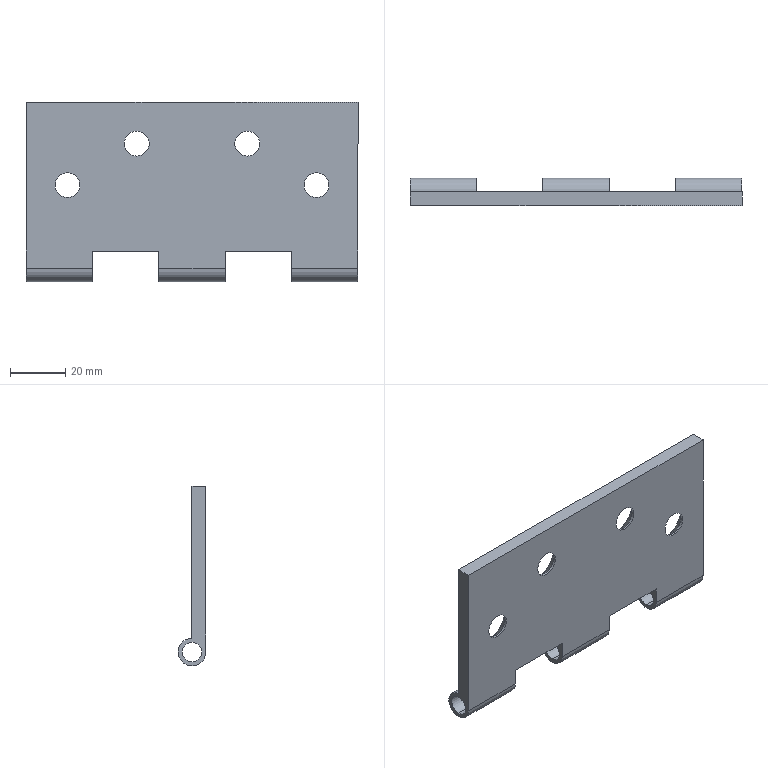Part | SolidWorks | features BaseBody 1 | 1 solid | 36 faces | box 120 x 10 x 65 mm | volume 33485 mm3 | cylinder 17 | plane 11 | cone 8 | commonest cylinder face diameters 9 x8 7 x6 10 x3
STEP:
#1=CARTESIAN_POINT('',(45.,0.85,-4.5));
#2=VERTEX_POINT('',#1);
#3=CARTESIAN_POINT('',(45.,0.85,4.5));
#4=VERTEX_POINT('',#3);
#5=CARTESIAN_POINT('',(45.,0.85,0.));
#6=DIRECTION('',(0.,1.,0.));
#7=DIRECTION('',(0.,0.,1.));
#8=AXIS2_PLACEMENT_3D('',#5,#6,#7);
#9=CIRCLE('',#8,4.5);
#10=EDGE_CURVE('',#2,#4,#9,.T.);
#11=ORIENTED_EDGE('',*,*,#10,.F.);
#12=CARTESIAN_POINT('',(45.,5.,-8.65));
#13=VERTEX_POINT('',#12);
#14=CARTESIAN_POINT('',(45.,5.,-8.65));
#15=DIRECTION('',(0.,0.7071,-0.7071));
#16=VECTOR('',#15,1000.);
#17=LINE('',#14,#16);
#18=EDGE_CURVE('',#2,#13,#17,.T.);
#19=ORIENTED_EDGE('',*,*,#18,.T.);
#20=CARTESIAN_POINT('',(45.,5.,8.65));
#21=VERTEX_POINT('',#20);
#22=CARTESIAN_POINT('',(45.,5.,0.));
#23=DIRECTION('',(0.,1.,0.));
#24=DIRECTION('',(0.,0.,1.));
#25=AXIS2_PLACEMENT_3D('',#22,#23,#24);
#26=CIRCLE('',#25,8.65);
#27=EDGE_CURVE('',#13,#21,#26,.T.);
#28=ORIENTED_EDGE('',*,*,#27,.T.);
#29=CARTESIAN_POINT('',(45.,5.,8.65));
#30=DIRECTION('',(0.,0.7071,0.7071));
#31=VECTOR('',#30,1000.);
#32=LINE('',#29,#31);
#33=EDGE_CURVE('',#4,#21,#32,.T.);
#34=ORIENTED_EDGE('',*,*,#33,.F.);
#35=EDGE_LOOP('',(#11,#19,#28,#34));
#36=FACE_OUTER_BOUND('',#35,.T.);
#37=CARTESIAN_POINT('',(45.,5.,0.));
#38=DIRECTION('',(0.,1.,0.));
#39=DIRECTION('',(0.,0.,1.));
#40=AXIS2_PLACEMENT_3D('',#37,#38,#39);
#41=CONICAL_SURFACE('',#40,8.65,0.7854);
#42=ADVANCED_FACE('',(#36),#41,.F.);
#43=CARTESIAN_POINT('',(45.,0.,-4.5));
#44=VERTEX_POINT('',#43);
#45=CARTESIAN_POINT('',(45.,0.,4.5));
#46=VERTEX_POINT('',#45);
#47=CARTESIAN_POINT('',(45.,0.,0.));
#48=DIRECTION('',(0.,1.,0.));
#49=DIRECTION('',(0.,0.,1.));
#50=AXIS2_PLACEMENT_3D('',#47,#48,#49);
#51=CIRCLE('',#50,4.5);
#52=EDGE_CURVE('',#44,#46,#51,.T.);
#53=ORIENTED_EDGE('',*,*,#52,.F.);
#54=CARTESIAN_POINT('',(45.,5.,-4.5));
#55=DIRECTION('',(0.,1.,0.));
#56=VECTOR('',#55,1000.);
#57=LINE('',#54,#56);
#58=EDGE_CURVE('',#44,#2,#57,.T.);
#59=ORIENTED_EDGE('',*,*,#58,.T.);
#60=ORIENTED_EDGE('',*,*,#10,.T.);
#61=CARTESIAN_POINT('',(45.,5.,4.5));
#62=DIRECTION('',(0.,1.,0.));
#63=VECTOR('',#62,1000.);
#64=LINE('',#61,#63);
#65=EDGE_CURVE('',#46,#4,#64,.T.);
#66=ORIENTED_EDGE('',*,*,#65,.F.);
#67=EDGE_LOOP('',(#53,#59,#60,#66));
#68=FACE_OUTER_BOUND('',#67,.T.);
#69=CARTESIAN_POINT('',(45.,5.,0.));
#70=DIRECTION('',(0.,1.,0.));
#71=DIRECTION('',(0.,0.,1.));
#72=AXIS2_PLACEMENT_3D('',#69,#70,#71);
#73=CYLINDRICAL_SURFACE('',#72,4.5);
#74=ADVANCED_FACE('',(#68),#73,.F.);
#75=CARTESIAN_POINT('',(20.,0.85,10.5));
#76=VERTEX_POINT('',#75);
#77=CARTESIAN_POINT('',(20.,0.85,19.5));
#78=VERTEX_POINT('',#77);
#79=CARTESIAN_POINT('',(20.,0.85,15.));
#80=DIRECTION('',(0.,1.,0.));
#81=DIRECTION('',(0.,0.,1.));
#82=AXIS2_PLACEMENT_3D('',#79,#80,#81);
#83=CIRCLE('',#82,4.5);
#84=EDGE_CURVE('',#76,#78,#83,.T.);
#85=ORIENTED_EDGE('',*,*,#84,.F.);
#86=CARTESIAN_POINT('',(20.,5.,6.35));
#87=VERTEX_POINT('',#86);
#88=CARTESIAN_POINT('',(20.,5.,6.35));
#89=DIRECTION('',(0.,0.7071,-0.7071));
#90=VECTOR('',#89,1000.);
#91=LINE('',#88,#90);
#92=EDGE_CURVE('',#76,#87,#91,.T.);
#93=ORIENTED_EDGE('',*,*,#92,.T.);
#94=CARTESIAN_POINT('',(20.,5.,23.65));
#95=VERTEX_POINT('',#94);
#96=CARTESIAN_POINT('',(20.,5.,15.));
#97=DIRECTION('',(0.,1.,0.));
#98=DIRECTION('',(0.,0.,1.));
#99=AXIS2_PLACEMENT_3D('',#96,#97,#98);
#100=CIRCLE('',#99,8.65);
#101=EDGE_CURVE('',#87,#95,#100,.T.);
#102=ORIENTED_EDGE('',*,*,#101,.T.);
#103=CARTESIAN_POINT('',(20.,5.,23.65));
#104=DIRECTION('',(0.,0.7071,0.7071));
#105=VECTOR('',#104,1000.);
#106=LINE('',#103,#105);
#107=EDGE_CURVE('',#78,#95,#106,.T.);
#108=ORIENTED_EDGE('',*,*,#107,.F.);
#109=EDGE_LOOP('',(#85,#93,#102,#108));
#110=FACE_OUTER_BOUND('',#109,.T.);
#111=CARTESIAN_POINT('',(20.,5.,15.));
#112=DIRECTION('',(0.,1.,0.));
#113=DIRECTION('',(0.,0.,1.));
#114=AXIS2_PLACEMENT_3D('',#111,#112,#113);
#115=CONICAL_SURFACE('',#114,8.65,0.7854);
#116=ADVANCED_FACE('',(#110),#115,.F.);
#117=CARTESIAN_POINT('',(20.,0.,10.5));
#118=VERTEX_POINT('',#117);
#119=CARTESIAN_POINT('',(20.,0.,19.5));
#120=VERTEX_POINT('',#119);
#121=CARTESIAN_POINT('',(20.,0.,15.));
#122=DIRECTION('',(0.,1.,0.));
#123=DIRECTION('',(0.,0.,1.));
#124=AXIS2_PLACEMENT_3D('',#121,#122,#123);
#125=CIRCLE('',#124,4.5);
#126=EDGE_CURVE('',#118,#120,#125,.T.);
#127=ORIENTED_EDGE('',*,*,#126,.F.);
#128=CARTESIAN_POINT('',(20.,5.,10.5));
#129=DIRECTION('',(0.,1.,0.));
#130=VECTOR('',#129,1000.);
#131=LINE('',#128,#130);
#132=EDGE_CURVE('',#118,#76,#131,.T.);
#133=ORIENTED_EDGE('',*,*,#132,.T.);
#134=ORIENTED_EDGE('',*,*,#84,.T.);
#135=CARTESIAN_POINT('',(20.,5.,19.5));
#136=DIRECTION('',(0.,1.,0.));
#137=VECTOR('',#136,1000.);
#138=LINE('',#135,#137);
#139=EDGE_CURVE('',#120,#78,#138,.T.);
#140=ORIENTED_EDGE('',*,*,#139,.F.);
#141=EDGE_LOOP('',(#127,#133,#134,#140));
#142=FACE_OUTER_BOUND('',#141,.T.);
#143=CARTESIAN_POINT('',(20.,5.,15.));
#144=DIRECTION('',(0.,1.,0.));
#145=DIRECTION('',(0.,0.,1.));
#146=AXIS2_PLACEMENT_3D('',#143,#144,#145);
#147=CYLINDRICAL_SURFACE('',#146,4.5);
#148=ADVANCED_FACE('',(#142),#147,.F.);
#149=CARTESIAN_POINT('',(-45.,0.85,-4.5));
#150=VERTEX_POINT('',#149);
#151=CARTESIAN_POINT('',(-45.,0.85,4.5));
#152=VERTEX_POINT('',#151);
#153=CARTESIAN_POINT('',(-45.,0.85,0.));
#154=DIRECTION('',(0.,1.,0.));
#155=DIRECTION('',(0.,0.,1.));
#156=AXIS2_PLACEMENT_3D('',#153,#154,#155);
#157=CIRCLE('',#156,4.5);
#158=EDGE_CURVE('',#150,#152,#157,.T.);
#159=ORIENTED_EDGE('',*,*,#158,.F.);
#160=CARTESIAN_POINT('',(-45.,5.,-8.65));
#161=VERTEX_POINT('',#160);
#162=CARTESIAN_POINT('',(-45.,5.,-8.65));
#163=DIRECTION('',(0.,0.7071,-0.7071));
#164=VECTOR('',#163,1000.);
#165=LINE('',#162,#164);
#166=EDGE_CURVE('',#150,#161,#165,.T.);
#167=ORIENTED_EDGE('',*,*,#166,.T.);
#168=CARTESIAN_POINT('',(-45.,5.,8.65));
#169=VERTEX_POINT('',#168);
#170=CARTESIAN_POINT('',(-45.,5.,0.));
#171=DIRECTION('',(0.,1.,0.));
#172=DIRECTION('',(0.,0.,1.));
#173=AXIS2_PLACEMENT_3D('',#170,#171,#172);
#174=CIRCLE('',#173,8.65);
#175=EDGE_CURVE('',#161,#169,#174,.T.);
#176=ORIENTED_EDGE('',*,*,#175,.T.);
#177=CARTESIAN_POINT('',(-45.,5.,8.65));
#178=DIRECTION('',(0.,0.7071,0.7071));
#179=VECTOR('',#178,1000.);
#180=LINE('',#177,#179);
#181=EDGE_CURVE('',#152,#169,#180,.T.);
#182=ORIENTED_EDGE('',*,*,#181,.F.);
#183=EDGE_LOOP('',(#159,#167,#176,#182));
#184=FACE_OUTER_BOUND('',#183,.T.);
#185=CARTESIAN_POINT('',(-45.,5.,0.));
#186=DIRECTION('',(0.,1.,0.));
#187=DIRECTION('',(0.,0.,1.));
#188=AXIS2_PLACEMENT_3D('',#185,#186,#187);
#189=CONICAL_SURFACE('',#188,8.65,0.7854);
#190=ADVANCED_FACE('',(#184),#189,.F.);
#191=CARTESIAN_POINT('',(-45.,0.,-4.5));
#192=VERTEX_POINT('',#191);
#193=CARTESIAN_POINT('',(-45.,0.,4.5));
#194=VERTEX_POINT('',#193);
#195=CARTESIAN_POINT('',(-45.,0.,0.));
#196=DIRECTION('',(0.,1.,0.));
#197=DIRECTION('',(0.,0.,1.));
#198=AXIS2_PLACEMENT_3D('',#195,#196,#197);
#199=CIRCLE('',#198,4.5);
#200=EDGE_CURVE('',#192,#194,#199,.T.);
#201=ORIENTED_EDGE('',*,*,#200,.F.);
#202=CARTESIAN_POINT('',(-45.,5.,-4.5));
#203=DIRECTION('',(0.,1.,0.));
#204=VECTOR('',#203,1000.);
#205=LINE('',#202,#204);
#206=EDGE_CURVE('',#192,#150,#205,.T.);
#207=ORIENTED_EDGE('',*,*,#206,.T.);
#208=ORIENTED_EDGE('',*,*,#158,.T.);
#209=CARTESIAN_POINT('',(-45.,5.,4.5));
#210=DIRECTION('',(0.,1.,0.));
#211=VECTOR('',#210,1000.);
#212=LINE('',#209,#211);
#213=EDGE_CURVE('',#194,#152,#212,.T.);
#214=ORIENTED_EDGE('',*,*,#213,.F.);
#215=EDGE_LOOP('',(#201,#207,#208,#214));
#216=FACE_OUTER_BOUND('',#215,.T.);
#217=CARTESIAN_POINT('',(-45.,5.,0.));
#218=DIRECTION('',(0.,1.,0.));
#219=DIRECTION('',(0.,0.,1.));
#220=AXIS2_PLACEMENT_3D('',#217,#218,#219);
#221=CYLINDRICAL_SURFACE('',#220,4.5);
#222=ADVANCED_FACE('',(#216),#221,.F.);
#223=CARTESIAN_POINT('',(-20.,0.85,10.5));
#224=VERTEX_POINT('',#223);
#225=CARTESIAN_POINT('',(-20.,0.85,19.5));
#226=VERTEX_POINT('',#225);
#227=CARTESIAN_POINT('',(-20.,0.85,15.));
#228=DIRECTION('',(0.,1.,0.));
#229=DIRECTION('',(0.,0.,1.));
#230=AXIS2_PLACEMENT_3D('',#227,#228,#229);
#231=CIRCLE('',#230,4.5);
#232=EDGE_CURVE('',#224,#226,#231,.T.);
#233=ORIENTED_EDGE('',*,*,#232,.F.);
#234=CARTESIAN_POINT('',(-20.,5.,6.35));
#235=VERTEX_POINT('',#234);
#236=CARTESIAN_POINT('',(-20.,5.,6.35));
#237=DIRECTION('',(0.,0.7071,-0.7071));
#238=VECTOR('',#237,1000.);
#239=LINE('',#236,#238);
#240=EDGE_CURVE('',#224,#235,#239,.T.);
#241=ORIENTED_EDGE('',*,*,#240,.T.);
#242=CARTESIAN_POINT('',(-20.,5.,23.65));
#243=VERTEX_POINT('',#242);
#244=CARTESIAN_POINT('',(-20.,5.,15.));
#245=DIRECTION('',(0.,1.,0.));
#246=DIRECTION('',(0.,0.,1.));
#247=AXIS2_PLACEMENT_3D('',#244,#245,#246);
#248=CIRCLE('',#247,8.65);
#249=EDGE_CURVE('',#235,#243,#248,.T.);
#250=ORIENTED_EDGE('',*,*,#249,.T.);
#251=CARTESIAN_POINT('',(-20.,5.,23.65));
#252=DIRECTION('',(0.,0.7071,0.7071));
#253=VECTOR('',#252,1000.);
#254=LINE('',#251,#253);
#255=EDGE_CURVE('',#226,#243,#254,.T.);
#256=ORIENTED_EDGE('',*,*,#255,.F.);
#257=EDGE_LOOP('',(#233,#241,#250,#256));
#258=FACE_OUTER_BOUND('',#257,.T.);
#259=CARTESIAN_POINT('',(-20.,5.,15.));
#260=DIRECTION('',(0.,1.,0.));
#261=DIRECTION('',(0.,0.,1.));
#262=AXIS2_PLACEMENT_3D('',#259,#260,#261);
#263=CONICAL_SURFACE('',#262,8.65,0.7854);
#264=ADVANCED_FACE('',(#258),#263,.F.);
#265=CARTESIAN_POINT('',(-20.,0.,10.5));
#266=VERTEX_POINT('',#265);
#267=CARTESIAN_POINT('',(-20.,0.,19.5));
#268=VERTEX_POINT('',#267);
#269=CARTESIAN_POINT('',(-20.,0.,15.));
#270=DIRECTION('',(0.,1.,0.));
#271=DIRECTION('',(0.,0.,1.));
#272=AXIS2_PLACEMENT_3D('',#269,#270,#271);
#273=CIRCLE('',#272,4.5);
#274=EDGE_CURVE('',#266,#268,#273,.T.);
#275=ORIENTED_EDGE('',*,*,#274,.F.);
#276=CARTESIAN_POINT('',(-20.,5.,10.5));
#277=DIRECTION('',(0.,1.,0.));
#278=VECTOR('',#277,1000.);
#279=LINE('',#276,#278);
#280=EDGE_CURVE('',#266,#224,#279,.T.);
#281=ORIENTED_EDGE('',*,*,#280,.T.);
#282=ORIENTED_EDGE('',*,*,#232,.T.);
#283=CARTESIAN_POINT('',(-20.,5.,19.5));
#284=DIRECTION('',(0.,1.,0.));
#285=VECTOR('',#284,1000.);
#286=LINE('',#283,#285);
#287=EDGE_CURVE('',#268,#226,#286,.T.);
#288=ORIENTED_EDGE('',*,*,#287,.F.);
#289=EDGE_LOOP('',(#275,#281,#282,#288));
#290=FACE_OUTER_BOUND('',#289,.T.);
#291=CARTESIAN_POINT('',(-20.,5.,15.));
#292=DIRECTION('',(0.,1.,0.));
#293=DIRECTION('',(0.,0.,1.));
#294=AXIS2_PLACEMENT_3D('',#291,#292,#293);
#295=CYLINDRICAL_SURFACE('',#294,4.5);
#296=ADVANCED_FACE('',(#290),#295,.F.);
#297=CARTESIAN_POINT('',(-36.,5.,-26.5));
#298=VERTEX_POINT('',#297);
#299=CARTESIAN_POINT('',(-36.,5.,-33.5));
#300=VERTEX_POINT('',#299);
#301=CARTESIAN_POINT('',(-36.,5.,-30.));
#302=DIRECTION('',(1.,0.,0.));
#303=DIRECTION('',(0.,0.,1.));
#304=AXIS2_PLACEMENT_3D('',#301,#302,#303);
#305=CIRCLE('',#304,3.5);
#306=EDGE_CURVE('',#298,#300,#305,.T.);
#307=ORIENTED_EDGE('',*,*,#306,.T.);
#308=CARTESIAN_POINT('',(-60.,5.,-33.5));
#309=VERTEX_POINT('',#308);
#310=CARTESIAN_POINT('',(60.,5.,-33.5));
#311=DIRECTION('',(-1.,0.,0.));
#312=VECTOR('',#311,1000.);
#313=LINE('',#310,#312);
#314=EDGE_CURVE('',#300,#309,#313,.T.);
#315=ORIENTED_EDGE('',*,*,#314,.T.);
#316=CARTESIAN_POINT('',(-60.,5.,-26.5));
#317=VERTEX_POINT('',#316);
#318=CARTESIAN_POINT('',(-60.,5.,-30.));
#319=DIRECTION('',(-1.,0.,0.));
#320=DIRECTION('',(0.,0.,1.));
#321=AXIS2_PLACEMENT_3D('',#318,#319,#320);
#322=CIRCLE('',#321,3.5);
#323=EDGE_CURVE('',#309,#317,#322,.T.);
#324=ORIENTED_EDGE('',*,*,#323,.T.);
#325=CARTESIAN_POINT('',(60.,5.,-26.5));
#326=DIRECTION('',(-1.,0.,0.));
#327=VECTOR('',#326,1000.);
#328=LINE('',#325,#327);
#329=EDGE_CURVE('',#298,#317,#328,.T.);
#330=ORIENTED_EDGE('',*,*,#329,.F.);
#331=EDGE_LOOP('',(#307,#315,#324,#330));
#332=FACE_OUTER_BOUND('',#331,.T.);
#333=CARTESIAN_POINT('',(60.,5.,-30.));
#334=DIRECTION('',(-1.,0.,0.));
#335=DIRECTION('',(0.,0.,1.));
#336=AXIS2_PLACEMENT_3D('',#333,#334,#335);
#337=CYLINDRICAL_SURFACE('',#336,3.5);
#338=ADVANCED_FACE('',(#332),#337,.F.);
#339=CARTESIAN_POINT('',(12.,5.,-26.5));
#340=VERTEX_POINT('',#339);
#341=CARTESIAN_POINT('',(12.,5.,-33.5));
#342=VERTEX_POINT('',#341);
#343=CARTESIAN_POINT('',(12.,5.,-30.));
#344=DIRECTION('',(1.,0.,0.));
#345=DIRECTION('',(0.,0.,1.));
#346=AXIS2_PLACEMENT_3D('',#343,#344,#345);
#347=CIRCLE('',#346,3.5);
#348=EDGE_CURVE('',#340,#342,#347,.T.);
#349=ORIENTED_EDGE('',*,*,#348,.T.);
#350=CARTESIAN_POINT('',(-12.,5.,-33.5));
#351=VERTEX_POINT('',#350);
#352=CARTESIAN_POINT('',(60.,5.,-33.5));
#353=DIRECTION('',(-1.,0.,0.));
#354=VECTOR('',#353,1000.);
#355=LINE('',#352,#354);
#356=EDGE_CURVE('',#342,#351,#355,.T.);
#357=ORIENTED_EDGE('',*,*,#356,.T.);
#358=CARTESIAN_POINT('',(-12.,5.,-26.5));
#359=VERTEX_POINT('',#358);
#360=CARTESIAN_POINT('',(-12.,5.,-30.));
#361=DIRECTION('',(-1.,0.,0.));
#362=DIRECTION('',(0.,0.,-1.));
#363=AXIS2_PLACEMENT_3D('',#360,#361,#362);
#364=CIRCLE('',#363,3.5);
#365=EDGE_CURVE('',#351,#359,#364,.T.);
#366=ORIENTED_EDGE('',*,*,#365,.T.);
#367=CARTESIAN_POINT('',(60.,5.,-26.5));
#368=DIRECTION('',(-1.,0.,0.));
#369=VECTOR('',#368,1000.);
#370=LINE('',#367,#369);
#371=EDGE_CURVE('',#340,#359,#370,.T.);
#372=ORIENTED_EDGE('',*,*,#371,.F.);
#373=EDGE_LOOP('',(#349,#357,#366,#372));
#374=FACE_OUTER_BOUND('',#373,.T.);
#375=CARTESIAN_POINT('',(60.,5.,-30.));
#376=DIRECTION('',(-1.,0.,0.));
#377=DIRECTION('',(0.,0.,1.));
#378=AXIS2_PLACEMENT_3D('',#375,#376,#377);
#379=CYLINDRICAL_SURFACE('',#378,3.5);
#380=ADVANCED_FACE('',(#374),#379,.F.);
#381=CARTESIAN_POINT('',(60.,5.,-33.5));
#382=VERTEX_POINT('',#381);
#383=CARTESIAN_POINT('',(60.,5.,-26.5));
#384=VERTEX_POINT('',#383);
#385=CARTESIAN_POINT('',(60.,5.,-30.));
#386=DIRECTION('',(-1.,0.,0.));
#387=DIRECTION('',(0.,0.,1.));
#388=AXIS2_PLACEMENT_3D('',#385,#386,#387);
#389=CIRCLE('',#388,3.5);
#390=EDGE_CURVE('',#382,#384,#389,.T.);
#391=ORIENTED_EDGE('',*,*,#390,.F.);
#392=CARTESIAN_POINT('',(36.,5.,-33.5));
#393=VERTEX_POINT('',#392);
#394=CARTESIAN_POINT('',(60.,5.,-33.5));
#395=DIRECTION('',(-1.,0.,0.));
#396=VECTOR('',#395,1000.);
#397=LINE('',#394,#396);
#398=EDGE_CURVE('',#382,#393,#397,.T.);
#399=ORIENTED_EDGE('',*,*,#398,.T.);
#400=CARTESIAN_POINT('',(36.,5.,-26.5));
#401=VERTEX_POINT('',#400);
#402=CARTESIAN_POINT('',(36.,5.,-30.));
#403=DIRECTION('',(-1.,0.,0.));
#404=DIRECTION('',(0.,0.,-1.));
#405=AXIS2_PLACEMENT_3D('',#402,#403,#404);
#406=CIRCLE('',#405,3.5);
#407=EDGE_CURVE('',#393,#401,#406,.T.);
#408=ORIENTED_EDGE('',*,*,#407,.T.);
#409=CARTESIAN_POINT('',(60.,5.,-26.5));
#410=DIRECTION('',(-1.,0.,0.));
#411=VECTOR('',#410,1000.);
#412=LINE('',#409,#411);
#413=EDGE_CURVE('',#384,#401,#412,.T.);
#414=ORIENTED_EDGE('',*,*,#413,.F.);
#415=EDGE_LOOP('',(#391,#399,#408,#414));
#416=FACE_OUTER_BOUND('',#415,.T.);
#417=CARTESIAN_POINT('',(60.,5.,-30.));
#418=DIRECTION('',(-1.,0.,0.));
#419=DIRECTION('',(0.,0.,1.));
#420=AXIS2_PLACEMENT_3D('',#417,#418,#419);
#421=CYLINDRICAL_SURFACE('',#420,3.5);
#422=ADVANCED_FACE('',(#416),#421,.F.);
#423=CARTESIAN_POINT('',(36.,5.,-25.));
#424=VERTEX_POINT('',#423);
#425=CARTESIAN_POINT('',(36.,0.,-30.));
#426=VERTEX_POINT('',#425);
#427=CARTESIAN_POINT('',(36.,5.,-30.));
#428=DIRECTION('',(-1.,0.,0.));
#429=DIRECTION('',(0.,0.,-1.));
#430=AXIS2_PLACEMENT_3D('',#427,#428,#429);
#431=CIRCLE('',#430,5.);
#432=EDGE_CURVE('',#424,#426,#431,.T.);
#433=ORIENTED_EDGE('',*,*,#432,.F.);
#434=CARTESIAN_POINT('',(60.,5.,-25.));
#435=VERTEX_POINT('',#434);
#436=CARTESIAN_POINT('',(60.,5.,-25.));
#437=DIRECTION('',(1.,0.,0.));
#438=VECTOR('',#437,1000.);
#439=LINE('',#436,#438);
#440=EDGE_CURVE('',#424,#435,#439,.T.);
#441=ORIENTED_EDGE('',*,*,#440,.T.);
#442=CARTESIAN_POINT('',(60.,0.,-30.));
#443=VERTEX_POINT('',#442);
#444=CARTESIAN_POINT('',(60.,5.,-30.));
#445=DIRECTION('',(-1.,0.,0.));
#446=DIRECTION('',(0.,0.,1.));
#447=AXIS2_PLACEMENT_3D('',#444,#445,#446);
#448=CIRCLE('',#447,5.);
#449=EDGE_CURVE('',#435,#443,#448,.T.);
#450=ORIENTED_EDGE('',*,*,#449,.T.);
#451=CARTESIAN_POINT('',(-60.,0.,-30.));
#452=DIRECTION('',(-1.,0.,0.));
#453=VECTOR('',#452,1000.);
#454=LINE('',#451,#453);
#455=EDGE_CURVE('',#443,#426,#454,.T.);
#456=ORIENTED_EDGE('',*,*,#455,.T.);
#457=EDGE_LOOP('',(#433,#441,#450,#456));
#458=FACE_OUTER_BOUND('',#457,.T.);
#459=CARTESIAN_POINT('',(60.,5.,-30.));
#460=DIRECTION('',(-1.,0.,0.));
#461=DIRECTION('',(0.,0.,1.));
#462=AXIS2_PLACEMENT_3D('',#459,#460,#461);
#463=CYLINDRICAL_SURFACE('',#462,5.);
#464=ADVANCED_FACE('',(#458),#463,.T.);
#465=ORIENTED_EDGE('',*,*,#398,.F.);
#466=CARTESIAN_POINT('',(60.,5.,-30.));
#467=DIRECTION('',(-1.,0.,0.));
#468=DIRECTION('',(0.,0.,1.));
#469=AXIS2_PLACEMENT_3D('',#466,#467,#468);
#470=CIRCLE('',#469,3.5);
#471=EDGE_CURVE('',#384,#382,#470,.T.);
#472=ORIENTED_EDGE('',*,*,#471,.F.);
#473=ORIENTED_EDGE('',*,*,#413,.T.);
#474=CARTESIAN_POINT('',(36.,5.,-30.));
#475=DIRECTION('',(-1.,0.,0.));
#476=DIRECTION('',(0.,0.,-1.));
#477=AXIS2_PLACEMENT_3D('',#474,#475,#476);
#478=CIRCLE('',#477,3.5);
#479=EDGE_CURVE('',#401,#393,#478,.T.);
#480=ORIENTED_EDGE('',*,*,#479,.T.);
#481=EDGE_LOOP('',(#465,#472,#473,#480));
#482=FACE_OUTER_BOUND('',#481,.T.);
#483=CARTESIAN_POINT('',(60.,5.,-30.));
#484=DIRECTION('',(-1.,0.,0.));
#485=DIRECTION('',(0.,0.,1.));
#486=AXIS2_PLACEMENT_3D('',#483,#484,#485);
#487=CYLINDRICAL_SURFACE('',#486,3.5);
#488=ADVANCED_FACE('',(#482),#487,.F.);
#489=CARTESIAN_POINT('',(12.,0.,-30.));
#490=VERTEX_POINT('',#489);
#491=CARTESIAN_POINT('',(12.,5.,-25.));
#492=VERTEX_POINT('',#491);
#493=CARTESIAN_POINT('',(12.,5.,-30.));
#494=DIRECTION('',(1.,0.,0.));
#495=DIRECTION('',(0.,0.,1.));
#496=AXIS2_PLACEMENT_3D('',#493,#494,#495);
#497=CIRCLE('',#496,5.);
#498=EDGE_CURVE('',#490,#492,#497,.T.);
#499=ORIENTED_EDGE('',*,*,#498,.F.);
#500=CARTESIAN_POINT('',(-12.,0.,-30.));
#501=VERTEX_POINT('',#500);
#502=CARTESIAN_POINT('',(-60.,0.,-30.));
#503=DIRECTION('',(-1.,0.,0.));
#504=VECTOR('',#503,1000.);
#505=LINE('',#502,#504);
#506=EDGE_CURVE('',#490,#501,#505,.T.);
#507=ORIENTED_EDGE('',*,*,#506,.T.);
#508=CARTESIAN_POINT('',(-12.,5.,-25.));
#509=VERTEX_POINT('',#508);
#510=CARTESIAN_POINT('',(-12.,5.,-30.));
#511=DIRECTION('',(-1.,0.,0.));
#512=DIRECTION('',(0.,0.,-1.));
#513=AXIS2_PLACEMENT_3D('',#510,#511,#512);
#514=CIRCLE('',#513,5.);
#515=EDGE_CURVE('',#509,#501,#514,.T.);
#516=ORIENTED_EDGE('',*,*,#515,.F.);
#517=CARTESIAN_POINT('',(60.,5.,-25.));
#518=DIRECTION('',(1.,0.,0.));
#519=VECTOR('',#518,1000.);
#520=LINE('',#517,#519);
#521=EDGE_CURVE('',#509,#492,#520,.T.);
#522=ORIENTED_EDGE('',*,*,#521,.T.);
#523=EDGE_LOOP('',(#499,#507,#516,#522));
#524=FACE_OUTER_BOUND('',#523,.T.);
#525=CARTESIAN_POINT('',(60.,5.,-30.));
#526=DIRECTION('',(-1.,0.,0.));
#527=DIRECTION('',(0.,0.,1.));
#528=AXIS2_PLACEMENT_3D('',#525,#526,#527);
#529=CYLINDRICAL_SURFACE('',#528,5.);
#530=ADVANCED_FACE('',(#524),#529,.T.);
#531=ORIENTED_EDGE('',*,*,#356,.F.);
#532=CARTESIAN_POINT('',(12.,5.,-30.));
#533=DIRECTION('',(1.,0.,0.));
#534=DIRECTION('',(0.,0.,1.));
#535=AXIS2_PLACEMENT_3D('',#532,#533,#534);
#536=CIRCLE('',#535,3.5);
#537=EDGE_CURVE('',#342,#340,#536,.T.);
#538=ORIENTED_EDGE('',*,*,#537,.T.);
#539=ORIENTED_EDGE('',*,*,#371,.T.);
#540=CARTESIAN_POINT('',(-12.,5.,-30.));
#541=DIRECTION('',(-1.,0.,0.));
#542=DIRECTION('',(0.,0.,-1.));
#543=AXIS2_PLACEMENT_3D('',#540,#541,#542);
#544=CIRCLE('',#543,3.5);
#545=EDGE_CURVE('',#359,#351,#544,.T.);
#546=ORIENTED_EDGE('',*,*,#545,.T.);
#547=EDGE_LOOP('',(#531,#538,#539,#546));
#548=FACE_OUTER_BOUND('',#547,.T.);
#549=CARTESIAN_POINT('',(60.,5.,-30.));
#550=DIRECTION('',(-1.,0.,0.));
#551=DIRECTION('',(0.,0.,1.));
#552=AXIS2_PLACEMENT_3D('',#549,#550,#551);
#553=CYLINDRICAL_SURFACE('',#552,3.5);
#554=ADVANCED_FACE('',(#548),#553,.F.);
#555=ORIENTED_EDGE('',*,*,#471,.T.);
#556=ORIENTED_EDGE('',*,*,#390,.T.);
#557=EDGE_LOOP('',(#555,#556));
#558=FACE_BOUND('',#557,.T.);
#559=CARTESIAN_POINT('',(60.,0.,30.));
#560=VERTEX_POINT('',#559);
#561=CARTESIAN_POINT('',(60.,0.,-30.));
#562=DIRECTION('',(0.,0.,-1.));
#563=VECTOR('',#562,1000.);
#564=LINE('',#561,#563);
#565=EDGE_CURVE('',#560,#443,#564,.T.);
#566=ORIENTED_EDGE('',*,*,#565,.T.);
#567=ORIENTED_EDGE('',*,*,#449,.F.);
#568=CARTESIAN_POINT('',(60.,5.,30.));
#569=VERTEX_POINT('',#568);
#570=CARTESIAN_POINT('',(60.,5.,-30.));
#571=DIRECTION('',(0.,0.,-1.));
#572=VECTOR('',#571,1000.);
#573=LINE('',#570,#572);
#574=EDGE_CURVE('',#569,#435,#573,.T.);
#575=ORIENTED_EDGE('',*,*,#574,.F.);
#576=CARTESIAN_POINT('',(60.,5.,30.));
#577=DIRECTION('',(0.,-1.,0.));
#578=VECTOR('',#577,1000.);
#579=LINE('',#576,#578);
#580=EDGE_CURVE('',#569,#560,#579,.T.);
#581=ORIENTED_EDGE('',*,*,#580,.T.);
#582=EDGE_LOOP('',(#566,#567,#575,#581));
#583=FACE_OUTER_BOUND('',#582,.T.);
#584=CARTESIAN_POINT('',(60.,5.,-30.));
#585=DIRECTION('',(-1.,0.,0.));
#586=DIRECTION('',(0.,0.,1.));
#587=AXIS2_PLACEMENT_3D('',#584,#585,#586);
#588=PLANE('',#587);
#589=ADVANCED_FACE('',(#558,#583),#588,.F.);
#590=CARTESIAN_POINT('',(-60.,5.,-30.));
#591=DIRECTION('',(-1.,0.,0.));
#592=DIRECTION('',(0.,0.,1.));
#593=AXIS2_PLACEMENT_3D('',#590,#591,#592);
#594=CIRCLE('',#593,3.5);
#595=EDGE_CURVE('',#317,#309,#594,.T.);
#596=ORIENTED_EDGE('',*,*,#595,.F.);
#597=ORIENTED_EDGE('',*,*,#323,.F.);
#598=EDGE_LOOP('',(#596,#597));
#599=FACE_BOUND('',#598,.T.);
#600=CARTESIAN_POINT('',(-60.,5.,-25.));
#601=VERTEX_POINT('',#600);
#602=CARTESIAN_POINT('',(-60.,0.,-30.));
#603=VERTEX_POINT('',#602);
#604=CARTESIAN_POINT('',(-60.,5.,-30.));
#605=DIRECTION('',(-1.,0.,0.));
#606=DIRECTION('',(0.,0.,1.));
#607=AXIS2_PLACEMENT_3D('',#604,#605,#606);
#608=CIRCLE('',#607,5.);
#609=EDGE_CURVE('',#601,#603,#608,.T.);
#610=ORIENTED_EDGE('',*,*,#609,.T.);
#611=CARTESIAN_POINT('',(-60.,0.,30.));
#612=VERTEX_POINT('',#611);
#613=CARTESIAN_POINT('',(-60.,0.,-30.));
#614=DIRECTION('',(0.,0.,1.));
#615=VECTOR('',#614,1000.);
#616=LINE('',#613,#615);
#617=EDGE_CURVE('',#603,#612,#616,.T.);
#618=ORIENTED_EDGE('',*,*,#617,.T.);
#619=CARTESIAN_POINT('',(-60.,5.,30.));
#620=VERTEX_POINT('',#619);
#621=CARTESIAN_POINT('',(-60.,5.,30.));
#622=DIRECTION('',(0.,-1.,0.));
#623=VECTOR('',#622,1000.);
#624=LINE('',#621,#623);
#625=EDGE_CURVE('',#620,#612,#624,.T.);
#626=ORIENTED_EDGE('',*,*,#625,.F.);
#627=CARTESIAN_POINT('',(-60.,5.,-30.));
#628=DIRECTION('',(0.,0.,1.));
#629=VECTOR('',#628,1000.);
#630=LINE('',#627,#629);
#631=EDGE_CURVE('',#601,#620,#630,.T.);
#632=ORIENTED_EDGE('',*,*,#631,.F.);
#633=EDGE_LOOP('',(#610,#618,#626,#632));
#634=FACE_OUTER_BOUND('',#633,.T.);
#635=CARTESIAN_POINT('',(-60.,5.,-30.));
#636=DIRECTION('',(1.,0.,0.));
#637=DIRECTION('',(0.,0.,-1.));
#638=AXIS2_PLACEMENT_3D('',#635,#636,#637);
#639=PLANE('',#638);
#640=ADVANCED_FACE('',(#599,#634),#639,.F.);
#641=CARTESIAN_POINT('',(-60.,0.,30.));
#642=DIRECTION('',(1.,0.,0.));
#643=VECTOR('',#642,1000.);
#644=LINE('',#641,#643);
#645=EDGE_CURVE('',#612,#560,#644,.T.);
#646=ORIENTED_EDGE('',*,*,#645,.T.);
#647=ORIENTED_EDGE('',*,*,#580,.F.);
#648=CARTESIAN_POINT('',(-60.,5.,30.));
#649=DIRECTION('',(1.,0.,0.));
#650=VECTOR('',#649,1000.);
#651=LINE('',#648,#650);
#652=EDGE_CURVE('',#620,#569,#651,.T.);
#653=ORIENTED_EDGE('',*,*,#652,.F.);
#654=ORIENTED_EDGE('',*,*,#625,.T.);
#655=EDGE_LOOP('',(#646,#647,#653,#654));
#656=FACE_OUTER_BOUND('',#655,.T.);
#657=CARTESIAN_POINT('',(-60.,5.,30.));
#658=DIRECTION('',(0.,0.,-1.));
#659=DIRECTION('',(-1.,0.,0.));
#660=AXIS2_PLACEMENT_3D('',#657,#658,#659);
#661=PLANE('',#660);
#662=ADVANCED_FACE('',(#656),#661,.F.);
#663=CARTESIAN_POINT('',(36.,5.,-24.));
#664=VERTEX_POINT('',#663);
#665=CARTESIAN_POINT('',(36.,5.,30.));
#666=DIRECTION('',(0.,0.,-1.));
#667=VECTOR('',#666,1000.);
#668=LINE('',#665,#667);
#669=EDGE_CURVE('',#664,#424,#668,.T.);
#670=ORIENTED_EDGE('',*,*,#669,.F.);
#671=CARTESIAN_POINT('',(12.,5.,-24.));
#672=VERTEX_POINT('',#671);
#673=CARTESIAN_POINT('',(60.,5.,-24.));
#674=DIRECTION('',(1.,0.,0.));
#675=VECTOR('',#674,1000.);
#676=LINE('',#673,#675);
#677=EDGE_CURVE('',#672,#664,#676,.T.);
#678=ORIENTED_EDGE('',*,*,#677,.F.);
#679=CARTESIAN_POINT('',(12.,5.,30.));
#680=DIRECTION('',(0.,0.,1.));
#681=VECTOR('',#680,1000.);
#682=LINE('',#679,#681);
#683=EDGE_CURVE('',#492,#672,#682,.T.);
#684=ORIENTED_EDGE('',*,*,#683,.F.);
#685=ORIENTED_EDGE('',*,*,#521,.F.);
#686=CARTESIAN_POINT('',(-12.,5.,-24.));
#687=VERTEX_POINT('',#686);
#688=CARTESIAN_POINT('',(-12.,5.,30.));
#689=DIRECTION('',(0.,0.,-1.));
#690=VECTOR('',#689,1000.);
#691=LINE('',#688,#690);
#692=EDGE_CURVE('',#687,#509,#691,.T.);
#693=ORIENTED_EDGE('',*,*,#692,.F.);
#694=CARTESIAN_POINT('',(-36.,5.,-24.));
#695=VERTEX_POINT('',#694);
#696=CARTESIAN_POINT('',(60.,5.,-24.));
#697=DIRECTION('',(1.,0.,0.));
#698=VECTOR('',#697,1000.);
#699=LINE('',#696,#698);
#700=EDGE_CURVE('',#695,#687,#699,.T.);
#701=ORIENTED_EDGE('',*,*,#700,.F.);
#702=CARTESIAN_POINT('',(-36.,5.,-25.));
#703=VERTEX_POINT('',#702);
#704=CARTESIAN_POINT('',(-36.,5.,30.));
#705=DIRECTION('',(0.,0.,1.));
#706=VECTOR('',#705,1000.);
#707=LINE('',#704,#706);
#708=EDGE_CURVE('',#703,#695,#707,.T.);
#709=ORIENTED_EDGE('',*,*,#708,.F.);
#710=CARTESIAN_POINT('',(60.,5.,-25.));
#711=DIRECTION('',(1.,0.,0.));
#712=VECTOR('',#711,1000.);
#713=LINE('',#710,#712);
#714=EDGE_CURVE('',#601,#703,#713,.T.);
#715=ORIENTED_EDGE('',*,*,#714,.F.);
#716=ORIENTED_EDGE('',*,*,#631,.T.);
#717=ORIENTED_EDGE('',*,*,#652,.T.);
#718=ORIENTED_EDGE('',*,*,#574,.T.);
#719=ORIENTED_EDGE('',*,*,#440,.F.);
#720=EDGE_LOOP('',(#670,#678,#684,#685,#693,#701,#709,#715,#716,#717,#718,#719));
#721=FACE_OUTER_BOUND('',#720,.T.);
#722=CARTESIAN_POINT('',(45.,5.,0.));
#723=DIRECTION('',(0.,1.,0.));
#724=DIRECTION('',(0.,0.,1.));
#725=AXIS2_PLACEMENT_3D('',#722,#723,#724);
#726=CIRCLE('',#725,8.65);
#727=EDGE_CURVE('',#21,#13,#726,.T.);
#728=ORIENTED_EDGE('',*,*,#727,.F.);
#729=ORIENTED_EDGE('',*,*,#27,.F.);
#730=EDGE_LOOP('',(#728,#729));
#731=FACE_BOUND('',#730,.T.);
#732=CARTESIAN_POINT('',(20.,5.,15.));
#733=DIRECTION('',(0.,1.,0.));
#734=DIRECTION('',(0.,0.,1.));
#735=AXIS2_PLACEMENT_3D('',#732,#733,#734);
#736=CIRCLE('',#735,8.65);
#737=EDGE_CURVE('',#95,#87,#736,.T.);
#738=ORIENTED_EDGE('',*,*,#737,.F.);
#739=ORIENTED_EDGE('',*,*,#101,.F.);
#740=EDGE_LOOP('',(#738,#739));
#741=FACE_BOUND('',#740,.T.);
#742=CARTESIAN_POINT('',(-45.,5.,0.));
#743=DIRECTION('',(0.,1.,0.));
#744=DIRECTION('',(0.,0.,1.));
#745=AXIS2_PLACEMENT_3D('',#742,#743,#744);
#746=CIRCLE('',#745,8.65);
#747=EDGE_CURVE('',#169,#161,#746,.T.);
#748=ORIENTED_EDGE('',*,*,#747,.F.);
#749=ORIENTED_EDGE('',*,*,#175,.F.);
#750=EDGE_LOOP('',(#748,#749));
#751=FACE_BOUND('',#750,.T.);
#752=CARTESIAN_POINT('',(-20.,5.,15.));
#753=DIRECTION('',(0.,1.,0.));
#754=DIRECTION('',(0.,0.,1.));
#755=AXIS2_PLACEMENT_3D('',#752,#753,#754);
#756=CIRCLE('',#755,8.65);
#757=EDGE_CURVE('',#243,#235,#756,.T.);
#758=ORIENTED_EDGE('',*,*,#757,.F.);
#759=ORIENTED_EDGE('',*,*,#249,.F.);
#760=EDGE_LOOP('',(#758,#759));
#761=FACE_BOUND('',#760,.T.);
#762=CARTESIAN_POINT('',(60.,5.,30.));
#763=DIRECTION('',(0.,1.,0.));
#764=DIRECTION('',(0.,0.,1.));
#765=AXIS2_PLACEMENT_3D('',#762,#763,#764);
#766=PLANE('',#765);
#767=ADVANCED_FACE('',(#721,#731,#741,#751,#761),#766,.T.);
#768=CARTESIAN_POINT('',(45.,0.,0.));
#769=DIRECTION('',(0.,1.,0.));
#770=DIRECTION('',(0.,0.,1.));
#771=AXIS2_PLACEMENT_3D('',#768,#769,#770);
#772=CIRCLE('',#771,4.5);
#773=EDGE_CURVE('',#46,#44,#772,.T.);
#774=ORIENTED_EDGE('',*,*,#773,.T.);
#775=ORIENTED_EDGE('',*,*,#52,.T.);
#776=EDGE_LOOP('',(#774,#775));
#777=FACE_BOUND('',#776,.T.);
#778=CARTESIAN_POINT('',(20.,0.,15.));
#779=DIRECTION('',(0.,1.,0.));
#780=DIRECTION('',(0.,0.,1.));
#781=AXIS2_PLACEMENT_3D('',#778,#779,#780);
#782=CIRCLE('',#781,4.5);
#783=EDGE_CURVE('',#120,#118,#782,.T.);
#784=ORIENTED_EDGE('',*,*,#783,.T.);
#785=ORIENTED_EDGE('',*,*,#126,.T.);
#786=EDGE_LOOP('',(#784,#785));
#787=FACE_BOUND('',#786,.T.);
#788=CARTESIAN_POINT('',(-45.,0.,0.));
#789=DIRECTION('',(0.,1.,0.));
#790=DIRECTION('',(0.,0.,1.));
#791=AXIS2_PLACEMENT_3D('',#788,#789,#790);
#792=CIRCLE('',#791,4.5);
#793=EDGE_CURVE('',#194,#192,#792,.T.);
#794=ORIENTED_EDGE('',*,*,#793,.T.);
#795=ORIENTED_EDGE('',*,*,#200,.T.);
#796=EDGE_LOOP('',(#794,#795));
#797=FACE_BOUND('',#796,.T.);
#798=CARTESIAN_POINT('',(-20.,0.,15.));
#799=DIRECTION('',(0.,1.,0.));
#800=DIRECTION('',(0.,0.,1.));
#801=AXIS2_PLACEMENT_3D('',#798,#799,#800);
#802=CIRCLE('',#801,4.5);
#803=EDGE_CURVE('',#268,#266,#802,.T.);
#804=ORIENTED_EDGE('',*,*,#803,.T.);
#805=ORIENTED_EDGE('',*,*,#274,.T.);
#806=EDGE_LOOP('',(#804,#805));
#807=FACE_BOUND('',#806,.T.);
#808=CARTESIAN_POINT('',(12.,0.,-24.));
#809=VERTEX_POINT('',#808);
#810=CARTESIAN_POINT('',(36.,0.,-24.));
#811=VERTEX_POINT('',#810);
#812=CARTESIAN_POINT('',(60.,0.,-24.));
#813=DIRECTION('',(1.,0.,0.));
#814=VECTOR('',#813,1000.);
#815=LINE('',#812,#814);
#816=EDGE_CURVE('',#809,#811,#815,.T.);
#817=ORIENTED_EDGE('',*,*,#816,.T.);
#818=CARTESIAN_POINT('',(36.,0.,30.));
#819=DIRECTION('',(0.,0.,-1.));
#820=VECTOR('',#819,1000.);
#821=LINE('',#818,#820);
#822=EDGE_CURVE('',#811,#426,#821,.T.);
#823=ORIENTED_EDGE('',*,*,#822,.T.);
#824=ORIENTED_EDGE('',*,*,#455,.F.);
#825=ORIENTED_EDGE('',*,*,#565,.F.);
#826=ORIENTED_EDGE('',*,*,#645,.F.);
#827=ORIENTED_EDGE('',*,*,#617,.F.);
#828=CARTESIAN_POINT('',(-36.,0.,-30.));
#829=VERTEX_POINT('',#828);
#830=CARTESIAN_POINT('',(-60.,0.,-30.));
#831=DIRECTION('',(-1.,0.,0.));
#832=VECTOR('',#831,1000.);
#833=LINE('',#830,#832);
#834=EDGE_CURVE('',#829,#603,#833,.T.);
#835=ORIENTED_EDGE('',*,*,#834,.F.);
#836=CARTESIAN_POINT('',(-36.,0.,-24.));
#837=VERTEX_POINT('',#836);
#838=CARTESIAN_POINT('',(-36.,0.,30.));
#839=DIRECTION('',(0.,0.,1.));
#840=VECTOR('',#839,1000.);
#841=LINE('',#838,#840);
#842=EDGE_CURVE('',#829,#837,#841,.T.);
#843=ORIENTED_EDGE('',*,*,#842,.T.);
#844=CARTESIAN_POINT('',(-12.,0.,-24.));
#845=VERTEX_POINT('',#844);
#846=CARTESIAN_POINT('',(60.,0.,-24.));
#847=DIRECTION('',(1.,0.,0.));
#848=VECTOR('',#847,1000.);
#849=LINE('',#846,#848);
#850=EDGE_CURVE('',#837,#845,#849,.T.);
#851=ORIENTED_EDGE('',*,*,#850,.T.);
#852=CARTESIAN_POINT('',(-12.,0.,30.));
#853=DIRECTION('',(0.,0.,-1.));
#854=VECTOR('',#853,1000.);
#855=LINE('',#852,#854);
#856=EDGE_CURVE('',#845,#501,#855,.T.);
#857=ORIENTED_EDGE('',*,*,#856,.T.);
#858=ORIENTED_EDGE('',*,*,#506,.F.);
#859=CARTESIAN_POINT('',(12.,0.,30.));
#860=DIRECTION('',(0.,0.,1.));
#861=VECTOR('',#860,1000.);
#862=LINE('',#859,#861);
#863=EDGE_CURVE('',#490,#809,#862,.T.);
#864=ORIENTED_EDGE('',*,*,#863,.T.);
#865=EDGE_LOOP('',(#817,#823,#824,#825,#826,#827,#835,#843,#851,#857,#858,#864));
#866=FACE_OUTER_BOUND('',#865,.T.);
#867=CARTESIAN_POINT('',(60.,0.,30.));
#868=DIRECTION('',(0.,1.,0.));
#869=DIRECTION('',(0.,0.,1.));
#870=AXIS2_PLACEMENT_3D('',#867,#868,#869);
#871=PLANE('',#870);
#872=ADVANCED_FACE('',(#777,#787,#797,#807,#866),#871,.F.);
#873=CARTESIAN_POINT('',(-36.,5.,-30.));
#874=DIRECTION('',(1.,0.,0.));
#875=DIRECTION('',(0.,0.,1.));
#876=AXIS2_PLACEMENT_3D('',#873,#874,#875);
#877=CIRCLE('',#876,5.);
#878=EDGE_CURVE('',#829,#703,#877,.T.);
#879=ORIENTED_EDGE('',*,*,#878,.F.);
#880=ORIENTED_EDGE('',*,*,#834,.T.);
#881=ORIENTED_EDGE('',*,*,#609,.F.);
#882=ORIENTED_EDGE('',*,*,#714,.T.);
#883=EDGE_LOOP('',(#879,#880,#881,#882));
#884=FACE_OUTER_BOUND('',#883,.T.);
#885=CARTESIAN_POINT('',(60.,5.,-30.));
#886=DIRECTION('',(-1.,0.,0.));
#887=DIRECTION('',(0.,0.,1.));
#888=AXIS2_PLACEMENT_3D('',#885,#886,#887);
#889=CYLINDRICAL_SURFACE('',#888,5.);
#890=ADVANCED_FACE('',(#884),#889,.T.);
#891=ORIENTED_EDGE('',*,*,#314,.F.);
#892=CARTESIAN_POINT('',(-36.,5.,-30.));
#893=DIRECTION('',(1.,0.,0.));
#894=DIRECTION('',(0.,0.,1.));
#895=AXIS2_PLACEMENT_3D('',#892,#893,#894);
#896=CIRCLE('',#895,3.5);
#897=EDGE_CURVE('',#300,#298,#896,.T.);
#898=ORIENTED_EDGE('',*,*,#897,.T.);
#899=ORIENTED_EDGE('',*,*,#329,.T.);
#900=ORIENTED_EDGE('',*,*,#595,.T.);
#901=EDGE_LOOP('',(#891,#898,#899,#900));
#902=FACE_OUTER_BOUND('',#901,.T.);
#903=CARTESIAN_POINT('',(60.,5.,-30.));
#904=DIRECTION('',(-1.,0.,0.));
#905=DIRECTION('',(0.,0.,1.));
#906=AXIS2_PLACEMENT_3D('',#903,#904,#905);
#907=CYLINDRICAL_SURFACE('',#906,3.5);
#908=ADVANCED_FACE('',(#902),#907,.F.);
#909=ORIENTED_EDGE('',*,*,#280,.F.);
#910=ORIENTED_EDGE('',*,*,#803,.F.);
#911=ORIENTED_EDGE('',*,*,#287,.T.);
#912=CARTESIAN_POINT('',(-20.,0.85,15.));
#913=DIRECTION('',(0.,1.,0.));
#914=DIRECTION('',(0.,0.,1.));
#915=AXIS2_PLACEMENT_3D('',#912,#913,#914);
#916=CIRCLE('',#915,4.5);
#917=EDGE_CURVE('',#226,#224,#916,.T.);
#918=ORIENTED_EDGE('',*,*,#917,.T.);
#919=EDGE_LOOP('',(#909,#910,#911,#918));
#920=FACE_OUTER_BOUND('',#919,.T.);
#921=CARTESIAN_POINT('',(-20.,5.,15.));
#922=DIRECTION('',(0.,1.,0.));
#923=DIRECTION('',(0.,0.,1.));
#924=AXIS2_PLACEMENT_3D('',#921,#922,#923);
#925=CYLINDRICAL_SURFACE('',#924,4.5);
#926=ADVANCED_FACE('',(#920),#925,.F.);
#927=ORIENTED_EDGE('',*,*,#240,.F.);
#928=ORIENTED_EDGE('',*,*,#917,.F.);
#929=ORIENTED_EDGE('',*,*,#255,.T.);
#930=ORIENTED_EDGE('',*,*,#757,.T.);
#931=EDGE_LOOP('',(#927,#928,#929,#930));
#932=FACE_OUTER_BOUND('',#931,.T.);
#933=CARTESIAN_POINT('',(-20.,5.,15.));
#934=DIRECTION('',(0.,1.,0.));
#935=DIRECTION('',(0.,0.,1.));
#936=AXIS2_PLACEMENT_3D('',#933,#934,#935);
#937=CONICAL_SURFACE('',#936,8.65,0.7854);
#938=ADVANCED_FACE('',(#932),#937,.F.);
#939=ORIENTED_EDGE('',*,*,#206,.F.);
#940=ORIENTED_EDGE('',*,*,#793,.F.);
#941=ORIENTED_EDGE('',*,*,#213,.T.);
#942=CARTESIAN_POINT('',(-45.,0.85,0.));
#943=DIRECTION('',(0.,1.,0.));
#944=DIRECTION('',(0.,0.,1.));
#945=AXIS2_PLACEMENT_3D('',#942,#943,#944);
#946=CIRCLE('',#945,4.5);
#947=EDGE_CURVE('',#152,#150,#946,.T.);
#948=ORIENTED_EDGE('',*,*,#947,.T.);
#949=EDGE_LOOP('',(#939,#940,#941,#948));
#950=FACE_OUTER_BOUND('',#949,.T.);
#951=CARTESIAN_POINT('',(-45.,5.,0.));
#952=DIRECTION('',(0.,1.,0.));
#953=DIRECTION('',(0.,0.,1.));
#954=AXIS2_PLACEMENT_3D('',#951,#952,#953);
#955=CYLINDRICAL_SURFACE('',#954,4.5);
#956=ADVANCED_FACE('',(#950),#955,.F.);
#957=ORIENTED_EDGE('',*,*,#166,.F.);
#958=ORIENTED_EDGE('',*,*,#947,.F.);
#959=ORIENTED_EDGE('',*,*,#181,.T.);
#960=ORIENTED_EDGE('',*,*,#747,.T.);
#961=EDGE_LOOP('',(#957,#958,#959,#960));
#962=FACE_OUTER_BOUND('',#961,.T.);
#963=CARTESIAN_POINT('',(-45.,5.,0.));
#964=DIRECTION('',(0.,1.,0.));
#965=DIRECTION('',(0.,0.,1.));
#966=AXIS2_PLACEMENT_3D('',#963,#964,#965);
#967=CONICAL_SURFACE('',#966,8.65,0.7854);
#968=ADVANCED_FACE('',(#962),#967,.F.);
#969=ORIENTED_EDGE('',*,*,#132,.F.);
#970=ORIENTED_EDGE('',*,*,#783,.F.);
#971=ORIENTED_EDGE('',*,*,#139,.T.);
#972=CARTESIAN_POINT('',(20.,0.85,15.));
#973=DIRECTION('',(0.,1.,0.));
#974=DIRECTION('',(0.,0.,1.));
#975=AXIS2_PLACEMENT_3D('',#972,#973,#974);
#976=CIRCLE('',#975,4.5);
#977=EDGE_CURVE('',#78,#76,#976,.T.);
#978=ORIENTED_EDGE('',*,*,#977,.T.);
#979=EDGE_LOOP('',(#969,#970,#971,#978));
#980=FACE_OUTER_BOUND('',#979,.T.);
#981=CARTESIAN_POINT('',(20.,5.,15.));
#982=DIRECTION('',(0.,1.,0.));
#983=DIRECTION('',(0.,0.,1.));
#984=AXIS2_PLACEMENT_3D('',#981,#982,#983);
#985=CYLINDRICAL_SURFACE('',#984,4.5);
#986=ADVANCED_FACE('',(#980),#985,.F.);
#987=ORIENTED_EDGE('',*,*,#92,.F.);
#988=ORIENTED_EDGE('',*,*,#977,.F.);
#989=ORIENTED_EDGE('',*,*,#107,.T.);
#990=ORIENTED_EDGE('',*,*,#737,.T.);
#991=EDGE_LOOP('',(#987,#988,#989,#990));
#992=FACE_OUTER_BOUND('',#991,.T.);
#993=CARTESIAN_POINT('',(20.,5.,15.));
#994=DIRECTION('',(0.,1.,0.));
#995=DIRECTION('',(0.,0.,1.));
#996=AXIS2_PLACEMENT_3D('',#993,#994,#995);
#997=CONICAL_SURFACE('',#996,8.65,0.7854);
#998=ADVANCED_FACE('',(#992),#997,.F.);
#999=ORIENTED_EDGE('',*,*,#58,.F.);
#1000=ORIENTED_EDGE('',*,*,#773,.F.);
#1001=ORIENTED_EDGE('',*,*,#65,.T.);
#1002=CARTESIAN_POINT('',(45.,0.85,0.));
#1003=DIRECTION('',(0.,1.,0.));
#1004=DIRECTION('',(0.,0.,1.));
#1005=AXIS2_PLACEMENT_3D('',#1002,#1003,#1004);
#1006=CIRCLE('',#1005,4.5);
#1007=EDGE_CURVE('',#4,#2,#1006,.T.);
#1008=ORIENTED_EDGE('',*,*,#1007,.T.);
#1009=EDGE_LOOP('',(#999,#1000,#1001,#1008));
#1010=FACE_OUTER_BOUND('',#1009,.T.);
#1011=CARTESIAN_POINT('',(45.,5.,0.));
#1012=DIRECTION('',(0.,1.,0.));
#1013=DIRECTION('',(0.,0.,1.));
#1014=AXIS2_PLACEMENT_3D('',#1011,#1012,#1013);
#1015=CYLINDRICAL_SURFACE('',#1014,4.5);
#1016=ADVANCED_FACE('',(#1010),#1015,.F.);
#1017=ORIENTED_EDGE('',*,*,#18,.F.);
#1018=ORIENTED_EDGE('',*,*,#1007,.F.);
#1019=ORIENTED_EDGE('',*,*,#33,.T.);
#1020=ORIENTED_EDGE('',*,*,#727,.T.);
#1021=EDGE_LOOP('',(#1017,#1018,#1019,#1020));
#1022=FACE_OUTER_BOUND('',#1021,.T.);
#1023=CARTESIAN_POINT('',(45.,5.,0.));
#1024=DIRECTION('',(0.,1.,0.));
#1025=DIRECTION('',(0.,0.,1.));
#1026=AXIS2_PLACEMENT_3D('',#1023,#1024,#1025);
#1027=CONICAL_SURFACE('',#1026,8.65,0.7854);
#1028=ADVANCED_FACE('',(#1022),#1027,.F.);
#1029=ORIENTED_EDGE('',*,*,#700,.T.);
#1030=CARTESIAN_POINT('',(-12.,-7.,-24.));
#1031=DIRECTION('',(0.,1.,0.));
#1032=VECTOR('',#1031,1000.);
#1033=LINE('',#1030,#1032);
#1034=EDGE_CURVE('',#845,#687,#1033,.T.);
#1035=ORIENTED_EDGE('',*,*,#1034,.F.);
#1036=ORIENTED_EDGE('',*,*,#850,.F.);
#1037=CARTESIAN_POINT('',(-36.,-7.,-24.));
#1038=DIRECTION('',(0.,1.,0.));
#1039=VECTOR('',#1038,1000.);
#1040=LINE('',#1037,#1039);
#1041=EDGE_CURVE('',#837,#695,#1040,.T.);
#1042=ORIENTED_EDGE('',*,*,#1041,.T.);
#1043=EDGE_LOOP('',(#1029,#1035,#1036,#1042));
#1044=FACE_OUTER_BOUND('',#1043,.T.);
#1045=CARTESIAN_POINT('',(-36.,-7.,-24.));
#1046=DIRECTION('',(0.,0.,1.));
#1047=DIRECTION('',(1.,0.,0.));
#1048=AXIS2_PLACEMENT_3D('',#1045,#1046,#1047);
#1049=PLANE('',#1048);
#1050=ADVANCED_FACE('',(#1044),#1049,.F.);
#1051=ORIENTED_EDGE('',*,*,#692,.T.);
#1052=ORIENTED_EDGE('',*,*,#515,.T.);
#1053=ORIENTED_EDGE('',*,*,#856,.F.);
#1054=ORIENTED_EDGE('',*,*,#1034,.T.);
#1055=EDGE_LOOP('',(#1051,#1052,#1053,#1054));
#1056=FACE_OUTER_BOUND('',#1055,.T.);
#1057=ORIENTED_EDGE('',*,*,#545,.F.);
#1058=ORIENTED_EDGE('',*,*,#365,.F.);
#1059=EDGE_LOOP('',(#1057,#1058));
#1060=FACE_BOUND('',#1059,.T.);
#1061=CARTESIAN_POINT('',(-12.,-7.,-36.));
#1062=DIRECTION('',(1.,0.,0.));
#1063=DIRECTION('',(0.,0.,-1.));
#1064=AXIS2_PLACEMENT_3D('',#1061,#1062,#1063);
#1065=PLANE('',#1064);
#1066=ADVANCED_FACE('',(#1056,#1060),#1065,.F.);
#1067=ORIENTED_EDGE('',*,*,#708,.T.);
#1068=ORIENTED_EDGE('',*,*,#1041,.F.);
#1069=ORIENTED_EDGE('',*,*,#842,.F.);
#1070=ORIENTED_EDGE('',*,*,#878,.T.);
#1071=EDGE_LOOP('',(#1067,#1068,#1069,#1070));
#1072=FACE_OUTER_BOUND('',#1071,.T.);
#1073=ORIENTED_EDGE('',*,*,#306,.F.);
#1074=ORIENTED_EDGE('',*,*,#897,.F.);
#1075=EDGE_LOOP('',(#1073,#1074));
#1076=FACE_BOUND('',#1075,.T.);
#1077=CARTESIAN_POINT('',(-36.,-7.,-36.));
#1078=DIRECTION('',(-1.,0.,0.));
#1079=DIRECTION('',(0.,0.,1.));
#1080=AXIS2_PLACEMENT_3D('',#1077,#1078,#1079);
#1081=PLANE('',#1080);
#1082=ADVANCED_FACE('',(#1072,#1076),#1081,.F.);
#1083=ORIENTED_EDGE('',*,*,#669,.T.);
#1084=ORIENTED_EDGE('',*,*,#432,.T.);
#1085=ORIENTED_EDGE('',*,*,#822,.F.);
#1086=CARTESIAN_POINT('',(36.,-7.,-24.));
#1087=DIRECTION('',(0.,1.,0.));
#1088=VECTOR('',#1087,1000.);
#1089=LINE('',#1086,#1088);
#1090=EDGE_CURVE('',#811,#664,#1089,.T.);
#1091=ORIENTED_EDGE('',*,*,#1090,.T.);
#1092=EDGE_LOOP('',(#1083,#1084,#1085,#1091));
#1093=FACE_OUTER_BOUND('',#1092,.T.);
#1094=ORIENTED_EDGE('',*,*,#479,.F.);
#1095=ORIENTED_EDGE('',*,*,#407,.F.);
#1096=EDGE_LOOP('',(#1094,#1095));
#1097=FACE_BOUND('',#1096,.T.);
#1098=CARTESIAN_POINT('',(36.,-7.,-36.));
#1099=DIRECTION('',(1.,0.,0.));
#1100=DIRECTION('',(0.,0.,-1.));
#1101=AXIS2_PLACEMENT_3D('',#1098,#1099,#1100);
#1102=PLANE('',#1101);
#1103=ADVANCED_FACE('',(#1093,#1097),#1102,.F.);
#1104=ORIENTED_EDGE('',*,*,#677,.T.);
#1105=ORIENTED_EDGE('',*,*,#1090,.F.);
#1106=ORIENTED_EDGE('',*,*,#816,.F.);
#1107=CARTESIAN_POINT('',(12.,-7.,-24.));
#1108=DIRECTION('',(0.,1.,0.));
#1109=VECTOR('',#1108,1000.);
#1110=LINE('',#1107,#1109);
#1111=EDGE_CURVE('',#809,#672,#1110,.T.);
#1112=ORIENTED_EDGE('',*,*,#1111,.T.);
#1113=EDGE_LOOP('',(#1104,#1105,#1106,#1112));
#1114=FACE_OUTER_BOUND('',#1113,.T.);
#1115=CARTESIAN_POINT('',(12.,-7.,-24.));
#1116=DIRECTION('',(0.,0.,1.));
#1117=DIRECTION('',(1.,0.,0.));
#1118=AXIS2_PLACEMENT_3D('',#1115,#1116,#1117);
#1119=PLANE('',#1118);
#1120=ADVANCED_FACE('',(#1114),#1119,.F.);
#1121=ORIENTED_EDGE('',*,*,#683,.T.);
#1122=ORIENTED_EDGE('',*,*,#1111,.F.);
#1123=ORIENTED_EDGE('',*,*,#863,.F.);
#1124=ORIENTED_EDGE('',*,*,#498,.T.);
#1125=EDGE_LOOP('',(#1121,#1122,#1123,#1124));
#1126=FACE_OUTER_BOUND('',#1125,.T.);
#1127=ORIENTED_EDGE('',*,*,#348,.F.);
#1128=ORIENTED_EDGE('',*,*,#537,.F.);
#1129=EDGE_LOOP('',(#1127,#1128));
#1130=FACE_BOUND('',#1129,.T.);
#1131=CARTESIAN_POINT('',(12.,-7.,-36.));
#1132=DIRECTION('',(-1.,0.,0.));
#1133=DIRECTION('',(0.,0.,1.));
#1134=AXIS2_PLACEMENT_3D('',#1131,#1132,#1133);
#1135=PLANE('',#1134);
#1136=ADVANCED_FACE('',(#1126,#1130),#1135,.F.);
#1137=CLOSED_SHELL('',(#42,#74,#116,#148,#190,#222,#264,#296,#338,#380,#422,#464,#488,#530,#554,#589,#640,#662,#767,#872,#890,#908,#926,#938,#956,#968,#986,#998,#1016,#1028,#1050,#1066,#1082,#1103,#1120,#1136));
#1138=MANIFOLD_SOLID_BREP('',#1137);
#1139=CARTESIAN_POINT('',(0.,0.,0.));
#1140=DIRECTION('',(0.,0.,1.));
#1141=DIRECTION('',(1.,0.,0.));
#1142=AXIS2_PLACEMENT_3D('',#1139,#1140,#1141);
#1143=(LENGTH_UNIT()NAMED_UNIT(*)SI_UNIT(.MILLI.,.METRE.));
#1144=UNCERTAINTY_MEASURE_WITH_UNIT(LENGTH_MEASURE(0.00001),#1143,'','');
#1145=(NAMED_UNIT(*)PLANE_ANGLE_UNIT()SI_UNIT($,.RADIAN.));
#1146=(NAMED_UNIT(*)SI_UNIT($,.STERADIAN.)SOLID_ANGLE_UNIT());
#1147=(GEOMETRIC_REPRESENTATION_CONTEXT(3)GLOBAL_UNCERTAINTY_ASSIGNED_CONTEXT((#1144))GLOBAL_UNIT_ASSIGNED_CONTEXT((#1143,#1145,#1146))REPRESENTATION_CONTEXT('',''));
#1148=ADVANCED_BREP_SHAPE_REPRESENTATION('',(#1138,#1142),#1147);